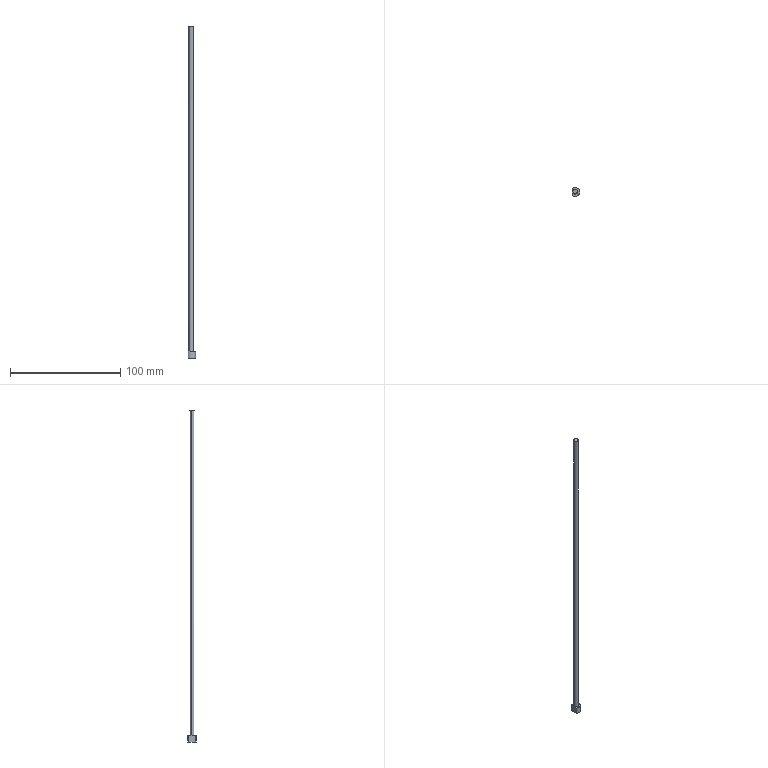Part | Creo | 1 solid | 7 faces | box 6.5 x 8 x 300.857 mm | volume 3965 mm3 | cylinder 3 | plane 3 | spline 1 | commonest cylinder face diameters 4 x2 8 x1
STEP:
#1=CARTESIAN_POINT('',(-59.,95.5,-290.));
#2=VERTEX_POINT('',#1);
#3=CARTESIAN_POINT('',(-63.,95.5,-290.));
#4=VERTEX_POINT('',#3);
#5=CARTESIAN_POINT('',(-61.,95.5,-290.));
#6=DIRECTION('',(0.,0.,-1.));
#7=DIRECTION('',(1.,0.,0.));
#8=AXIS2_PLACEMENT_3D('',#5,#6,#7);
#9=CIRCLE('',#8,2.);
#10=EDGE_CURVE('',#2,#4,#9,.T.);
#11=ORIENTED_EDGE('',*,*,#10,.T.);
#12=CARTESIAN_POINT('',(-63.,95.5,4.713));
#13=VERTEX_POINT('',#12);
#14=CARTESIAN_POINT('',(-63.,95.5,4.713));
#15=DIRECTION('',(0.000000002,-0.000000011,-1.));
#16=VECTOR('',#15,294.713);
#17=LINE('',#14,#16);
#18=EDGE_CURVE('',#13,#4,#17,.T.);
#19=ORIENTED_EDGE('',*,*,#18,.F.);
#20=CARTESIAN_POINT('',(-62.907,94.896,4.672));
#21=VERTEX_POINT('',#20);
#22=CARTESIAN_POINT('',(-62.937,94.993,4.678));
#23=CARTESIAN_POINT('',(-62.984,95.193,4.692));
#24=CARTESIAN_POINT('',(-63.,95.398,4.706));
#25=CARTESIAN_POINT('',(-63.,95.5,4.713));
#26=B_SPLINE_CURVE_WITH_KNOTS('',3,(#20,#22,#23,#24,#25),.UNSPECIFIED.,.F.,.F.,(4,1,4),(0.,0.5,1.),.UNSPECIFIED.);
#27=EDGE_CURVE('',#21,#13,#26,.T.);
#28=ORIENTED_EDGE('',*,*,#27,.F.);
#29=CARTESIAN_POINT('',(-59.,95.5,4.704));
#30=VERTEX_POINT('',#29);
#31=CARTESIAN_POINT('',(-62.907,94.896,4.672));
#32=CARTESIAN_POINT('',(-62.841,94.69,4.659));
#33=CARTESIAN_POINT('',(-62.646,94.304,4.634));
#34=CARTESIAN_POINT('',(-62.188,93.85,4.609));
#35=CARTESIAN_POINT('',(-61.626,93.566,4.596));
#36=CARTESIAN_POINT('',(-61.002,93.467,4.593));
#37=CARTESIAN_POINT('',(-60.37,93.566,4.599));
#38=CARTESIAN_POINT('',(-59.802,93.858,4.615));
#39=CARTESIAN_POINT('',(-59.357,94.304,4.638));
#40=CARTESIAN_POINT('',(-59.069,94.863,4.667));
#41=CARTESIAN_POINT('',(-59.,95.287,4.692));
#42=CARTESIAN_POINT('',(-59.,95.5,4.704));
#43=B_SPLINE_CURVE_WITH_KNOTS('',3,(#31,#32,#33,#34,#35,#36,#37,#38,#39,#40,#41,#42),.UNSPECIFIED.,.F.,.F.,(4,1,1,1,1,1,1,1,1,4),(0.,0.1111,0.2222,0.3333,0.4444,0.5556,0.6667,0.7778,0.8889,1.),.UNSPECIFIED.);
#44=EDGE_CURVE('',#21,#30,#43,.T.);
#45=ORIENTED_EDGE('',*,*,#44,.T.);
#46=CARTESIAN_POINT('',(-59.,95.5,4.704));
#47=DIRECTION('',(0.000000396,0.000000002,-1.));
#48=VECTOR('',#47,294.704);
#49=LINE('',#46,#48);
#50=EDGE_CURVE('',#30,#2,#49,.T.);
#51=ORIENTED_EDGE('',*,*,#50,.T.);
#52=EDGE_LOOP('',(#11,#19,#28,#45,#51));
#53=FACE_OUTER_BOUND('',#52,.F.);
#54=CARTESIAN_POINT('',(-61.,95.5,-5.));
#55=DIRECTION('',(0.,0.,-1.));
#56=DIRECTION('',(1.,0.,0.));
#57=AXIS2_PLACEMENT_3D('',#54,#55,#56);
#58=CYLINDRICAL_SURFACE('',#57,2.);
#59=ADVANCED_FACE('',(#53),#58,.T.);
#60=CARTESIAN_POINT('',(-63.5,98.622,-290.));
#61=VERTEX_POINT('',#60);
#62=CARTESIAN_POINT('',(-63.5,92.378,-290.));
#63=VERTEX_POINT('',#62);
#64=CARTESIAN_POINT('',(-63.5,98.622,-290.));
#65=DIRECTION('',(0.,-1.,0.));
#66=VECTOR('',#65,6.245);
#67=LINE('',#64,#66);
#68=EDGE_CURVE('',#61,#63,#67,.T.);
#69=ORIENTED_EDGE('',*,*,#68,.F.);
#70=CARTESIAN_POINT('',(-57.,95.5,-290.));
#71=VERTEX_POINT('',#70);
#72=CARTESIAN_POINT('',(-61.,95.5,-290.));
#73=DIRECTION('',(0.,0.,1.));
#74=DIRECTION('',(1.,0.,0.));
#75=AXIS2_PLACEMENT_3D('',#72,#73,#74);
#76=CIRCLE('',#75,4.);
#77=EDGE_CURVE('',#71,#61,#76,.T.);
#78=ORIENTED_EDGE('',*,*,#77,.F.);
#79=CARTESIAN_POINT('',(-61.,95.5,-290.));
#80=DIRECTION('',(0.,0.,1.));
#81=DIRECTION('',(-0.625,-0.7806,0.));
#82=AXIS2_PLACEMENT_3D('',#79,#80,#81);
#83=CIRCLE('',#82,4.);
#84=EDGE_CURVE('',#63,#71,#83,.T.);
#85=ORIENTED_EDGE('',*,*,#84,.F.);
#86=EDGE_LOOP('',(#69,#78,#85));
#87=FACE_OUTER_BOUND('',#86,.F.);
#88=ORIENTED_EDGE('',*,*,#10,.F.);
#89=CARTESIAN_POINT('',(-61.,95.5,-290.));
#90=DIRECTION('',(0.,0.,-1.));
#91=DIRECTION('',(-1.,0.,0.));
#92=AXIS2_PLACEMENT_3D('',#89,#90,#91);
#93=CIRCLE('',#92,2.);
#94=EDGE_CURVE('',#4,#2,#93,.T.);
#95=ORIENTED_EDGE('',*,*,#94,.F.);
#96=EDGE_LOOP('',(#88,#95));
#97=FACE_BOUND('',#96,.F.);
#98=CARTESIAN_POINT('',(-61.,95.5,-290.));
#99=DIRECTION('',(0.,0.,1.));
#100=DIRECTION('',(-1.,0.,0.));
#101=AXIS2_PLACEMENT_3D('',#98,#99,#100);
#102=PLANE('',#101);
#103=ADVANCED_FACE('',(#87,#97),#102,.T.);
#104=CARTESIAN_POINT('',(-63.5,98.622,-296.));
#105=VERTEX_POINT('',#104);
#106=CARTESIAN_POINT('',(-63.5,98.622,-296.));
#107=DIRECTION('',(0.,0.,1.));
#108=VECTOR('',#107,6.);
#109=LINE('',#106,#108);
#110=EDGE_CURVE('',#105,#61,#109,.T.);
#111=ORIENTED_EDGE('',*,*,#110,.T.);
#112=ORIENTED_EDGE('',*,*,#68,.T.);
#113=CARTESIAN_POINT('',(-63.5,92.378,-296.));
#114=VERTEX_POINT('',#113);
#115=CARTESIAN_POINT('',(-63.5,92.378,-290.));
#116=DIRECTION('',(0.,0.,-1.));
#117=VECTOR('',#116,6.);
#118=LINE('',#115,#117);
#119=EDGE_CURVE('',#63,#114,#118,.T.);
#120=ORIENTED_EDGE('',*,*,#119,.T.);
#121=CARTESIAN_POINT('',(-63.5,98.622,-296.));
#122=DIRECTION('',(0.,-1.,0.));
#123=VECTOR('',#122,6.245);
#124=LINE('',#121,#123);
#125=EDGE_CURVE('',#105,#114,#124,.T.);
#126=ORIENTED_EDGE('',*,*,#125,.F.);
#127=EDGE_LOOP('',(#111,#112,#120,#126));
#128=FACE_OUTER_BOUND('',#127,.F.);
#129=CARTESIAN_POINT('',(-63.5,95.5,-296.));
#130=DIRECTION('',(1.,0.,0.));
#131=DIRECTION('',(0.,0.,-1.));
#132=AXIS2_PLACEMENT_3D('',#129,#130,#131);
#133=PLANE('',#132);
#134=ADVANCED_FACE('',(#128),#133,.F.);
#135=ORIENTED_EDGE('',*,*,#110,.F.);
#136=CARTESIAN_POINT('',(-57.,95.5,-296.));
#137=VERTEX_POINT('',#136);
#138=CARTESIAN_POINT('',(-61.,95.5,-296.));
#139=DIRECTION('',(0.,0.,-1.));
#140=DIRECTION('',(-0.625,0.7806,0.));
#141=AXIS2_PLACEMENT_3D('',#138,#139,#140);
#142=CIRCLE('',#141,4.);
#143=EDGE_CURVE('',#105,#137,#142,.T.);
#144=ORIENTED_EDGE('',*,*,#143,.T.);
#145=CARTESIAN_POINT('',(-61.,95.5,-296.));
#146=DIRECTION('',(0.,0.,-1.));
#147=DIRECTION('',(1.,0.,0.));
#148=AXIS2_PLACEMENT_3D('',#145,#146,#147);
#149=CIRCLE('',#148,4.);
#150=EDGE_CURVE('',#137,#114,#149,.T.);
#151=ORIENTED_EDGE('',*,*,#150,.T.);
#152=ORIENTED_EDGE('',*,*,#119,.F.);
#153=ORIENTED_EDGE('',*,*,#84,.T.);
#154=ORIENTED_EDGE('',*,*,#77,.T.);
#155=EDGE_LOOP('',(#135,#144,#151,#152,#153,#154));
#156=FACE_OUTER_BOUND('',#155,.F.);
#157=CARTESIAN_POINT('',(-61.,95.5,-296.));
#158=DIRECTION('',(0.,0.,1.));
#159=DIRECTION('',(-1.,0.,0.));
#160=AXIS2_PLACEMENT_3D('',#157,#158,#159);
#161=CYLINDRICAL_SURFACE('',#160,4.);
#162=ADVANCED_FACE('',(#156),#161,.T.);
#163=ORIENTED_EDGE('',*,*,#150,.F.);
#164=ORIENTED_EDGE('',*,*,#143,.F.);
#165=ORIENTED_EDGE('',*,*,#125,.T.);
#166=EDGE_LOOP('',(#163,#164,#165));
#167=FACE_OUTER_BOUND('',#166,.F.);
#168=CARTESIAN_POINT('',(7.7,2.155,-296.));
#169=DIRECTION('',(0.,0.,1.));
#170=DIRECTION('',(0.,-1.,0.));
#171=AXIS2_PLACEMENT_3D('',#168,#169,#170);
#172=PLANE('',#171);
#173=ADVANCED_FACE('',(#167),#172,.F.);
#174=ORIENTED_EDGE('',*,*,#94,.T.);
#175=ORIENTED_EDGE('',*,*,#50,.F.);
#176=CARTESIAN_POINT('',(-59.094,96.104,4.743));
#177=VERTEX_POINT('',#176);
#178=CARTESIAN_POINT('',(-59.073,96.039,4.738));
#179=CARTESIAN_POINT('',(-59.038,95.907,4.73));
#180=CARTESIAN_POINT('',(-59.007,95.705,4.717));
#181=CARTESIAN_POINT('',(-59.,95.568,4.709));
#182=CARTESIAN_POINT('',(-59.,95.5,4.704));
#183=B_SPLINE_CURVE_WITH_KNOTS('',3,(#176,#178,#179,#180,#181,#182),.UNSPECIFIED.,.F.,.F.,(4,1,1,4),(0.,0.3333,0.6667,1.),.UNSPECIFIED.);
#184=EDGE_CURVE('',#177,#30,#183,.T.);
#185=ORIENTED_EDGE('',*,*,#184,.F.);
#186=CARTESIAN_POINT('',(-63.,95.5,4.713));
#187=CARTESIAN_POINT('',(-63.,95.712,4.728));
#188=CARTESIAN_POINT('',(-62.932,96.133,4.759));
#189=CARTESIAN_POINT('',(-62.644,96.695,4.801));
#190=CARTESIAN_POINT('',(-62.195,97.145,4.835));
#191=CARTESIAN_POINT('',(-61.627,97.434,4.855));
#192=CARTESIAN_POINT('',(-60.999,97.533,4.859));
#193=CARTESIAN_POINT('',(-60.371,97.433,4.846));
#194=CARTESIAN_POINT('',(-59.804,97.145,4.819));
#195=CARTESIAN_POINT('',(-59.347,96.685,4.783));
#196=CARTESIAN_POINT('',(-59.157,96.304,4.756));
#197=CARTESIAN_POINT('',(-59.094,96.104,4.743));
#198=B_SPLINE_CURVE_WITH_KNOTS('',3,(#186,#187,#188,#189,#190,#191,#192,#193,#194,#195,#196,#197),.UNSPECIFIED.,.F.,.F.,(4,1,1,1,1,1,1,1,1,4),(0.,0.1111,0.2222,0.3333,0.4444,0.5556,0.6667,0.7778,0.8889,1.),.UNSPECIFIED.);
#199=EDGE_CURVE('',#13,#177,#198,.T.);
#200=ORIENTED_EDGE('',*,*,#199,.F.);
#201=ORIENTED_EDGE('',*,*,#18,.T.);
#202=EDGE_LOOP('',(#174,#175,#185,#200,#201));
#203=FACE_OUTER_BOUND('',#202,.F.);
#204=CARTESIAN_POINT('',(-61.,95.5,-5.));
#205=DIRECTION('',(0.,0.,-1.));
#206=DIRECTION('',(1.,0.,0.));
#207=AXIS2_PLACEMENT_3D('',#204,#205,#206);
#208=CYLINDRICAL_SURFACE('',#207,2.);
#209=ADVANCED_FACE('',(#203),#208,.T.);
#210=ORIENTED_EDGE('',*,*,#27,.T.);
#211=ORIENTED_EDGE('',*,*,#199,.T.);
#212=ORIENTED_EDGE('',*,*,#184,.T.);
#213=ORIENTED_EDGE('',*,*,#44,.F.);
#214=EDGE_LOOP('',(#210,#211,#212,#213));
#215=FACE_OUTER_BOUND('',#214,.F.);
#216=CARTESIAN_POINT('',(-63.743,97.15,4.848));
#217=CARTESIAN_POINT('',(-63.306,95.628,4.711));
#218=CARTESIAN_POINT('',(-62.868,94.102,4.611));
#219=CARTESIAN_POINT('',(-62.431,92.575,4.548));
#220=CARTESIAN_POINT('',(-62.488,97.518,4.869));
#221=CARTESIAN_POINT('',(-62.047,96.003,4.733));
#222=CARTESIAN_POINT('',(-61.606,94.485,4.633));
#223=CARTESIAN_POINT('',(-61.166,92.966,4.569));
#224=CARTESIAN_POINT('',(-61.104,97.933,4.894));
#225=CARTESIAN_POINT('',(-60.659,96.427,4.758));
#226=CARTESIAN_POINT('',(-60.214,94.918,4.658));
#227=CARTESIAN_POINT('',(-59.769,93.407,4.594));
#228=CARTESIAN_POINT('',(-59.726,98.359,4.919));
#229=CARTESIAN_POINT('',(-59.276,96.862,4.784));
#230=CARTESIAN_POINT('',(-58.826,95.363,4.684));
#231=CARTESIAN_POINT('',(-58.377,93.862,4.621));
#232=CARTESIAN_POINT('',(-59.594,98.399,4.922));
#233=CARTESIAN_POINT('',(-59.144,96.904,4.786));
#234=CARTESIAN_POINT('',(-58.694,95.406,4.687));
#235=CARTESIAN_POINT('',(-58.243,93.906,4.623));
#236=B_SPLINE_SURFACE_WITH_KNOTS('',3,3,((#216,#217,#218,#219),(#220,#221,#222,#223),(#224,#225,#226,#227),(#228,#229,#230,#231),(#232,#233,#234,#235)),.UNSPECIFIED.,.F.,.F.,.F.,(4,1,4),(4,4),(0.3035,0.6492,0.6857),(0.2904,0.8414),.UNSPECIFIED.);
#237=ADVANCED_FACE('',(#215),#236,.F.);
#238=CLOSED_SHELL('',(#59,#103,#134,#162,#173,#209,#237));
#239=MANIFOLD_SOLID_BREP('',#238);
#240=(LENGTH_UNIT()NAMED_UNIT(*)SI_UNIT(.MILLI.,.METRE.));
#241=UNCERTAINTY_MEASURE_WITH_UNIT(LENGTH_MEASURE(0.03014),#240,'','');
#242=(NAMED_UNIT(*)PLANE_ANGLE_UNIT()SI_UNIT($,.RADIAN.));
#243=PLANE_ANGLE_MEASURE_WITH_UNIT(PLANE_ANGLE_MEASURE(0.01745),#242);
#244=(CONVERSION_BASED_UNIT('DEGREE',#243)NAMED_UNIT(*)PLANE_ANGLE_UNIT());
#245=(NAMED_UNIT(*)SI_UNIT($,.STERADIAN.)SOLID_ANGLE_UNIT());
#246=(GEOMETRIC_REPRESENTATION_CONTEXT(3)GLOBAL_UNCERTAINTY_ASSIGNED_CONTEXT((#241))GLOBAL_UNIT_ASSIGNED_CONTEXT((#240,#244,#245))REPRESENTATION_CONTEXT('',''));
#247=ADVANCED_BREP_SHAPE_REPRESENTATION('',(#239),#246);